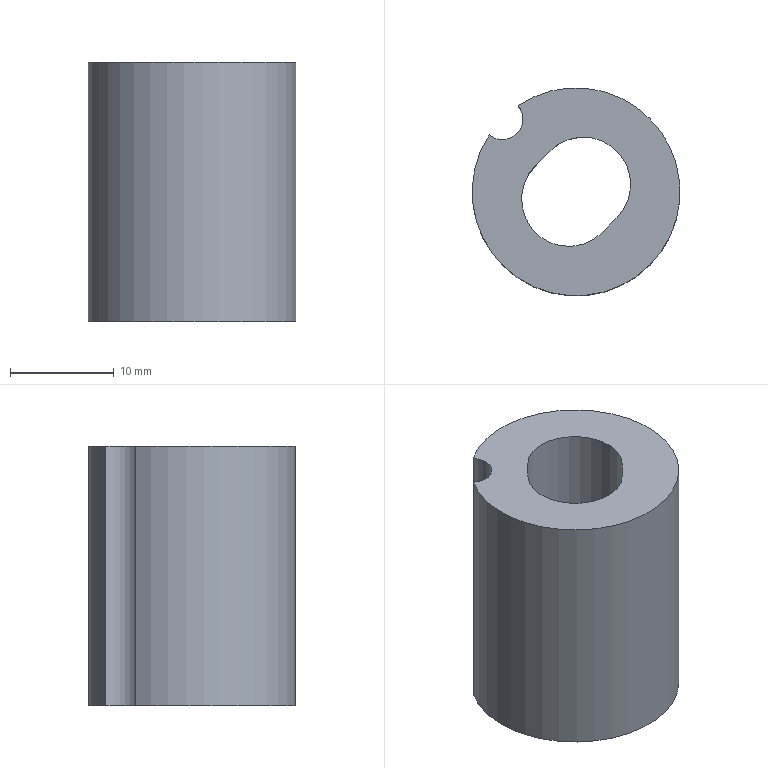Part | NX | features solid 2 | 1 solid | 10 faces | box 20 x 20 x 25 mm | volume 4918 mm3 | cylinder 5 | plane 5 | commonest cylinder face diameters 9.1 x2 4 x1 12.6 x1 20 x1
STEP:
#1=CARTESIAN_POINT('',(-363.871,534.082,-35.));
#2=VERTEX_POINT('',#1);
#3=CARTESIAN_POINT('',(-363.871,534.082,-10.));
#4=VERTEX_POINT('',#3);
#5=CARTESIAN_POINT('',(-363.871,534.082,-22.5));
#6=DIRECTION('',(0.,0.,1.));
#7=VECTOR('',#6,1000.);
#8=LINE('',#5,#7);
#9=EDGE_CURVE('',#2,#4,#8,.T.);
#10=ORIENTED_EDGE('',*,*,#9,.T.);
#11=CARTESIAN_POINT('',(-366.668,531.25,-10.));
#12=VERTEX_POINT('',#11);
#13=CARTESIAN_POINT('',(-358.298,525.779,-10.));
#14=DIRECTION('',(0.,0.,-1.));
#15=DIRECTION('',(-0.7114,0.7028,0.));
#16=AXIS2_PLACEMENT_3D('',#13,#14,#15);
#17=CIRCLE('',#16,10.);
#18=EDGE_CURVE('',#4,#12,#17,.T.);
#19=ORIENTED_EDGE('',*,*,#18,.T.);
#20=CARTESIAN_POINT('',(-366.668,531.25,-35.));
#21=VERTEX_POINT('',#20);
#22=CARTESIAN_POINT('',(-366.668,531.25,-22.5));
#23=DIRECTION('',(0.,0.,1.));
#24=VECTOR('',#23,1000.);
#25=LINE('',#22,#24);
#26=EDGE_CURVE('',#12,#21,#25,.F.);
#27=ORIENTED_EDGE('',*,*,#26,.T.);
#28=CARTESIAN_POINT('',(-358.298,525.779,-35.));
#29=DIRECTION('',(0.,0.,-1.));
#30=DIRECTION('',(-0.7114,0.7028,0.));
#31=AXIS2_PLACEMENT_3D('',#28,#29,#30);
#32=CIRCLE('',#31,10.);
#33=EDGE_CURVE('',#2,#21,#32,.T.);
#34=ORIENTED_EDGE('',*,*,#33,.F.);
#35=EDGE_LOOP('',(#10,#19,#27,#34));
#36=FACE_BOUND('',#35,.T.);
#37=CARTESIAN_POINT('',(-358.298,525.779,-35.));
#38=DIRECTION('',(0.,0.,1.));
#39=DIRECTION('',(-0.7114,0.7028,0.));
#40=AXIS2_PLACEMENT_3D('',#37,#38,#39);
#41=CYLINDRICAL_SURFACE('',#40,10.);
#42=ADVANCED_FACE('',(#36),#41,.T.);
#43=CARTESIAN_POINT('',(-362.779,530.206,-35.));
#44=VERTEX_POINT('',#43);
#45=CARTESIAN_POINT('',(-358.298,525.779,-35.));
#46=DIRECTION('',(0.,0.,-1.));
#47=DIRECTION('',(-0.7114,0.7028,0.));
#48=AXIS2_PLACEMENT_3D('',#45,#46,#47);
#49=CIRCLE('',#48,6.3);
#50=EDGE_CURVE('',#44,#44,#49,.T.);
#51=ORIENTED_EDGE('',*,*,#50,.F.);
#52=EDGE_LOOP('',(#51));
#53=FACE_BOUND('',#52,.T.);
#54=ORIENTED_EDGE('',*,*,#33,.T.);
#55=CARTESIAN_POINT('',(-365.412,532.807,-35.));
#56=DIRECTION('',(0.,0.,-1.));
#57=DIRECTION('',(-0.7114,0.7028,0.));
#58=AXIS2_PLACEMENT_3D('',#55,#56,#57);
#59=CIRCLE('',#58,2.);
#60=EDGE_CURVE('',#2,#21,#59,.T.);
#61=ORIENTED_EDGE('',*,*,#60,.F.);
#62=EDGE_LOOP('',(#54,#61));
#63=FACE_BOUND('',#62,.T.);
#64=CARTESIAN_POINT('',(-358.298,525.779,-35.));
#65=DIRECTION('',(0.,0.,1.));
#66=DIRECTION('',(-0.7114,0.7028,0.));
#67=AXIS2_PLACEMENT_3D('',#64,#65,#66);
#68=PLANE('',#67);
#69=ADVANCED_FACE('',(#53,#63),#68,.F.);
#70=CARTESIAN_POINT('',(-354.358,523.293,-10.));
#71=VERTEX_POINT('',#70);
#72=CARTESIAN_POINT('',(-355.763,521.87,-10.));
#73=VERTEX_POINT('',#72);
#74=CARTESIAN_POINT('',(-354.358,523.293,-10.));
#75=DIRECTION('',(-0.7028,-0.7114,0.));
#76=VECTOR('',#75,1000.);
#77=LINE('',#74,#76);
#78=EDGE_CURVE('',#71,#73,#77,.T.);
#79=ORIENTED_EDGE('',*,*,#78,.T.);
#80=CARTESIAN_POINT('',(-362.237,528.265,-10.));
#81=VERTEX_POINT('',#80);
#82=CARTESIAN_POINT('',(-359.,525.067,-10.));
#83=DIRECTION('',(0.,0.,-1.));
#84=DIRECTION('',(-0.7114,0.7028,0.));
#85=AXIS2_PLACEMENT_3D('',#82,#83,#84);
#86=CIRCLE('',#85,4.55);
#87=EDGE_CURVE('',#73,#81,#86,.T.);
#88=ORIENTED_EDGE('',*,*,#87,.T.);
#89=CARTESIAN_POINT('',(-360.832,529.688,-10.));
#90=VERTEX_POINT('',#89);
#91=CARTESIAN_POINT('',(-360.832,529.688,-10.));
#92=DIRECTION('',(-0.7028,-0.7114,0.));
#93=VECTOR('',#92,1000.);
#94=LINE('',#91,#93);
#95=EDGE_CURVE('',#90,#81,#94,.T.);
#96=ORIENTED_EDGE('',*,*,#95,.F.);
#97=CARTESIAN_POINT('',(-357.595,526.49,-10.));
#98=DIRECTION('',(0.,0.,-1.));
#99=DIRECTION('',(-0.7114,0.7028,0.));
#100=AXIS2_PLACEMENT_3D('',#97,#98,#99);
#101=CIRCLE('',#100,4.55);
#102=EDGE_CURVE('',#90,#71,#101,.T.);
#103=ORIENTED_EDGE('',*,*,#102,.T.);
#104=EDGE_LOOP('',(#79,#88,#96,#103));
#105=FACE_BOUND('',#104,.T.);
#106=CARTESIAN_POINT('',(-365.412,532.807,-10.));
#107=DIRECTION('',(0.,0.,-1.));
#108=DIRECTION('',(-0.7114,0.7028,0.));
#109=AXIS2_PLACEMENT_3D('',#106,#107,#108);
#110=CIRCLE('',#109,2.);
#111=EDGE_CURVE('',#4,#12,#110,.T.);
#112=ORIENTED_EDGE('',*,*,#111,.T.);
#113=ORIENTED_EDGE('',*,*,#18,.F.);
#114=EDGE_LOOP('',(#112,#113));
#115=FACE_BOUND('',#114,.T.);
#116=CARTESIAN_POINT('',(-358.298,525.779,-10.));
#117=DIRECTION('',(0.,0.,1.));
#118=DIRECTION('',(-0.7114,0.7028,0.));
#119=AXIS2_PLACEMENT_3D('',#116,#117,#118);
#120=PLANE('',#119);
#121=ADVANCED_FACE('',(#105,#115),#120,.T.);
#122=ORIENTED_EDGE('',*,*,#50,.T.);
#123=EDGE_LOOP('',(#122));
#124=FACE_BOUND('',#123,.T.);
#125=CARTESIAN_POINT('',(-362.779,530.206,-18.));
#126=VERTEX_POINT('',#125);
#127=CARTESIAN_POINT('',(-358.298,525.779,-18.));
#128=DIRECTION('',(0.,0.,-1.));
#129=DIRECTION('',(-0.7114,0.7028,0.));
#130=AXIS2_PLACEMENT_3D('',#127,#128,#129);
#131=CIRCLE('',#130,6.3);
#132=EDGE_CURVE('',#126,#126,#131,.T.);
#133=ORIENTED_EDGE('',*,*,#132,.F.);
#134=EDGE_LOOP('',(#133));
#135=FACE_BOUND('',#134,.T.);
#136=CARTESIAN_POINT('',(-358.298,525.779,-35.));
#137=DIRECTION('',(0.,0.,1.));
#138=DIRECTION('',(-0.7114,0.7028,0.));
#139=AXIS2_PLACEMENT_3D('',#136,#137,#138);
#140=CYLINDRICAL_SURFACE('',#139,6.3);
#141=ADVANCED_FACE('',(#124,#135),#140,.F.);
#142=CARTESIAN_POINT('',(-360.832,529.688,-18.));
#143=VERTEX_POINT('',#142);
#144=CARTESIAN_POINT('',(-354.358,523.293,-18.));
#145=VERTEX_POINT('',#144);
#146=CARTESIAN_POINT('',(-357.595,526.49,-18.));
#147=DIRECTION('',(0.,0.,-1.));
#148=DIRECTION('',(-0.7114,0.7028,0.));
#149=AXIS2_PLACEMENT_3D('',#146,#147,#148);
#150=CIRCLE('',#149,4.55);
#151=EDGE_CURVE('',#143,#145,#150,.T.);
#152=ORIENTED_EDGE('',*,*,#151,.F.);
#153=CARTESIAN_POINT('',(-362.237,528.265,-18.));
#154=VERTEX_POINT('',#153);
#155=CARTESIAN_POINT('',(-361.534,528.977,-18.));
#156=DIRECTION('',(-0.7028,-0.7114,0.));
#157=VECTOR('',#156,1000.);
#158=LINE('',#155,#157);
#159=EDGE_CURVE('',#143,#154,#158,.T.);
#160=ORIENTED_EDGE('',*,*,#159,.T.);
#161=CARTESIAN_POINT('',(-355.763,521.87,-18.));
#162=VERTEX_POINT('',#161);
#163=CARTESIAN_POINT('',(-359.,525.067,-18.));
#164=DIRECTION('',(0.,0.,-1.));
#165=DIRECTION('',(-0.7114,0.7028,0.));
#166=AXIS2_PLACEMENT_3D('',#163,#164,#165);
#167=CIRCLE('',#166,4.55);
#168=EDGE_CURVE('',#162,#154,#167,.T.);
#169=ORIENTED_EDGE('',*,*,#168,.F.);
#170=CARTESIAN_POINT('',(-355.061,522.581,-18.));
#171=DIRECTION('',(-0.7028,-0.7114,0.));
#172=VECTOR('',#171,1000.);
#173=LINE('',#170,#172);
#174=EDGE_CURVE('',#145,#162,#173,.T.);
#175=ORIENTED_EDGE('',*,*,#174,.F.);
#176=EDGE_LOOP('',(#152,#160,#169,#175));
#177=FACE_BOUND('',#176,.T.);
#178=ORIENTED_EDGE('',*,*,#132,.T.);
#179=EDGE_LOOP('',(#178));
#180=FACE_BOUND('',#179,.T.);
#181=CARTESIAN_POINT('',(-358.298,525.779,-18.));
#182=DIRECTION('',(0.,0.,1.));
#183=DIRECTION('',(-0.7114,0.7028,0.));
#184=AXIS2_PLACEMENT_3D('',#181,#182,#183);
#185=PLANE('',#184);
#186=ADVANCED_FACE('',(#177,#180),#185,.F.);
#187=ORIENTED_EDGE('',*,*,#9,.F.);
#188=ORIENTED_EDGE('',*,*,#60,.T.);
#189=ORIENTED_EDGE('',*,*,#26,.F.);
#190=ORIENTED_EDGE('',*,*,#111,.F.);
#191=EDGE_LOOP('',(#187,#188,#189,#190));
#192=FACE_BOUND('',#191,.T.);
#193=CARTESIAN_POINT('',(-365.412,532.807,-35.));
#194=DIRECTION('',(0.,0.,1.));
#195=DIRECTION('',(-0.7114,0.7028,0.));
#196=AXIS2_PLACEMENT_3D('',#193,#194,#195);
#197=CYLINDRICAL_SURFACE('',#196,2.);
#198=ADVANCED_FACE('',(#192),#197,.F.);
#199=CARTESIAN_POINT('',(-354.358,523.293,-35.));
#200=DIRECTION('',(0.,0.,1.));
#201=VECTOR('',#200,1000.);
#202=LINE('',#199,#201);
#203=EDGE_CURVE('',#145,#71,#202,.T.);
#204=ORIENTED_EDGE('',*,*,#203,.F.);
#205=ORIENTED_EDGE('',*,*,#174,.T.);
#206=CARTESIAN_POINT('',(-355.763,521.87,-35.));
#207=DIRECTION('',(0.,0.,1.));
#208=VECTOR('',#207,1000.);
#209=LINE('',#206,#208);
#210=EDGE_CURVE('',#162,#73,#209,.T.);
#211=ORIENTED_EDGE('',*,*,#210,.T.);
#212=ORIENTED_EDGE('',*,*,#78,.F.);
#213=EDGE_LOOP('',(#204,#205,#211,#212));
#214=FACE_BOUND('',#213,.T.);
#215=CARTESIAN_POINT('',(-354.358,523.293,-35.));
#216=DIRECTION('',(0.7114,-0.7028,0.));
#217=DIRECTION('',(0.,0.,1.));
#218=AXIS2_PLACEMENT_3D('',#215,#216,#217);
#219=PLANE('',#218);
#220=ADVANCED_FACE('',(#214),#219,.F.);
#221=ORIENTED_EDGE('',*,*,#210,.F.);
#222=ORIENTED_EDGE('',*,*,#168,.T.);
#223=CARTESIAN_POINT('',(-362.237,528.265,-35.));
#224=DIRECTION('',(0.,0.,1.));
#225=VECTOR('',#224,1000.);
#226=LINE('',#223,#225);
#227=EDGE_CURVE('',#154,#81,#226,.T.);
#228=ORIENTED_EDGE('',*,*,#227,.T.);
#229=ORIENTED_EDGE('',*,*,#87,.F.);
#230=EDGE_LOOP('',(#221,#222,#228,#229));
#231=FACE_BOUND('',#230,.T.);
#232=CARTESIAN_POINT('',(-359.,525.067,-35.));
#233=DIRECTION('',(0.,0.,1.));
#234=DIRECTION('',(-0.7114,0.7028,0.));
#235=AXIS2_PLACEMENT_3D('',#232,#233,#234);
#236=CYLINDRICAL_SURFACE('',#235,4.55);
#237=ADVANCED_FACE('',(#231),#236,.F.);
#238=ORIENTED_EDGE('',*,*,#159,.F.);
#239=CARTESIAN_POINT('',(-360.832,529.688,-35.));
#240=DIRECTION('',(0.,0.,1.));
#241=VECTOR('',#240,1000.);
#242=LINE('',#239,#241);
#243=EDGE_CURVE('',#143,#90,#242,.T.);
#244=ORIENTED_EDGE('',*,*,#243,.T.);
#245=ORIENTED_EDGE('',*,*,#95,.T.);
#246=ORIENTED_EDGE('',*,*,#227,.F.);
#247=EDGE_LOOP('',(#238,#244,#245,#246));
#248=FACE_BOUND('',#247,.T.);
#249=CARTESIAN_POINT('',(-360.832,529.688,-35.));
#250=DIRECTION('',(0.7114,-0.7028,0.));
#251=DIRECTION('',(0.,0.,1.));
#252=AXIS2_PLACEMENT_3D('',#249,#250,#251);
#253=PLANE('',#252);
#254=ADVANCED_FACE('',(#248),#253,.T.);
#255=ORIENTED_EDGE('',*,*,#243,.F.);
#256=ORIENTED_EDGE('',*,*,#151,.T.);
#257=ORIENTED_EDGE('',*,*,#203,.T.);
#258=ORIENTED_EDGE('',*,*,#102,.F.);
#259=EDGE_LOOP('',(#255,#256,#257,#258));
#260=FACE_BOUND('',#259,.T.);
#261=CARTESIAN_POINT('',(-357.595,526.49,-35.));
#262=DIRECTION('',(0.,0.,1.));
#263=DIRECTION('',(-0.7114,0.7028,0.));
#264=AXIS2_PLACEMENT_3D('',#261,#262,#263);
#265=CYLINDRICAL_SURFACE('',#264,4.55);
#266=ADVANCED_FACE('',(#260),#265,.F.);
#267=CLOSED_SHELL('',(#42,#69,#121,#141,#186,#198,#220,#237,#254,#266));
#268=MANIFOLD_SOLID_BREP('',#267);
#269=(LENGTH_UNIT()NAMED_UNIT(*)SI_UNIT(.MILLI.,.METRE.));
#270=UNCERTAINTY_MEASURE_WITH_UNIT(LENGTH_MEASURE(0.00001),#269,'','');
#271=(NAMED_UNIT(*)PLANE_ANGLE_UNIT()SI_UNIT($,.RADIAN.));
#272=(NAMED_UNIT(*)SI_UNIT($,.STERADIAN.)SOLID_ANGLE_UNIT());
#273=(GEOMETRIC_REPRESENTATION_CONTEXT(3)GLOBAL_UNCERTAINTY_ASSIGNED_CONTEXT((#270))GLOBAL_UNIT_ASSIGNED_CONTEXT((#269,#271,#272))REPRESENTATION_CONTEXT('',''));
#274=ADVANCED_BREP_SHAPE_REPRESENTATION('',(#268),#273);